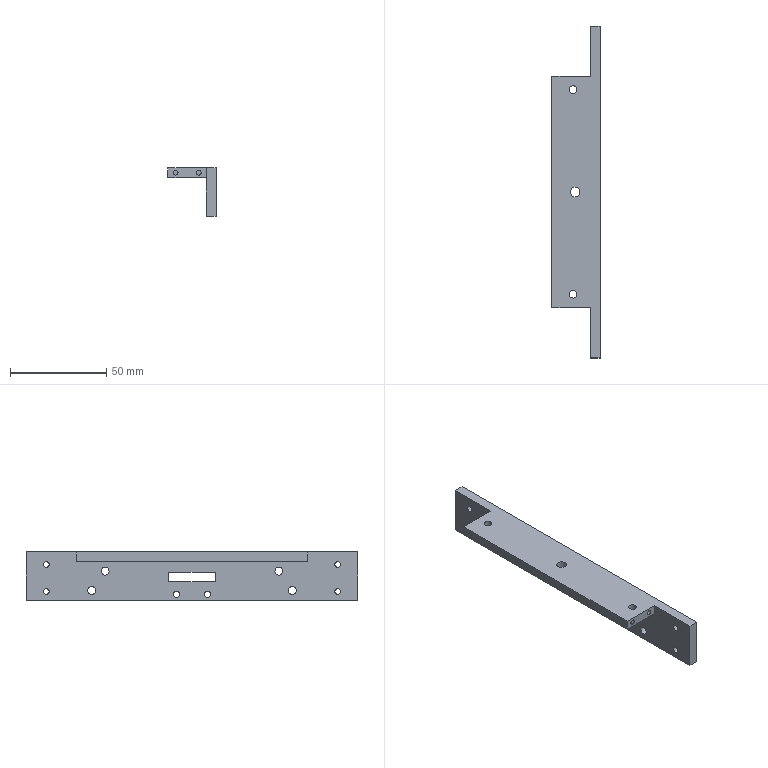Part | STEP file | 1-40.2 | 1 solid | 35 faces | box 25 x 172 x 25 mm | volume 31997 mm3 | plane 18 | cylinder 17 | commonest cylinder face diameters 3 x6 4 x6 2.5 x4 5 x1